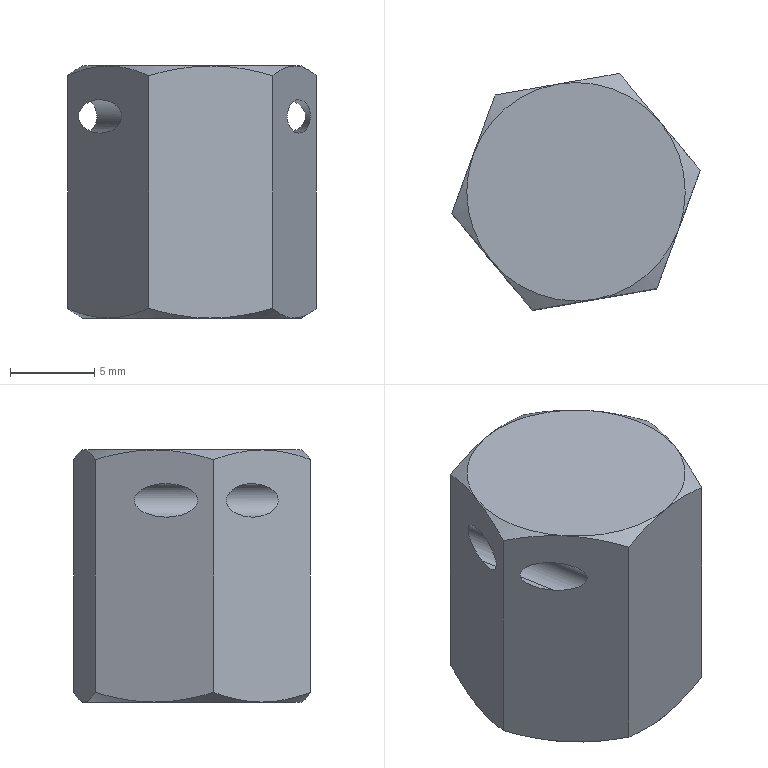Part | SolidWorks | features BaseBody 1 | 1 solid | 24 faces | box 14.79 x 14.092 x 15 mm | volume 2158 mm3 | cone 12 | plane 8 | cylinder 4 | commonest cylinder face diameters 2 x4
STEP:
#1=CARTESIAN_POINT('',(-50.82,56.44,-257.05));
#2=VERTEX_POINT('',#1);
#3=CARTESIAN_POINT('',(-50.82,56.44,-255.05));
#4=VERTEX_POINT('',#3);
#5=CARTESIAN_POINT('',(-50.82,56.44,-257.05));
#6=CARTESIAN_POINT('',(-49.442,60.195,-257.05));
#7=CARTESIAN_POINT('',(-49.442,60.195,-255.05));
#8=CARTESIAN_POINT('',(-50.82,56.44,-255.05));
#9=(BOUNDED_CURVE()B_SPLINE_CURVE(3,(#5,#6,#7,#8),.UNSPECIFIED.,.F.,.F.)B_SPLINE_CURVE_WITH_KNOTS((4,4),(1.571,4.712),.UNSPECIFIED.)CURVE()GEOMETRIC_REPRESENTATION_ITEM()RATIONAL_B_SPLINE_CURVE((1.,0.3333,0.3333,1.))REPRESENTATION_ITEM(''));
#10=EDGE_CURVE('',#2,#4,#9,.T.);
#11=ORIENTED_EDGE('',*,*,#10,.F.);
#12=CARTESIAN_POINT('',(-49.929,51.301,-257.05));
#13=VERTEX_POINT('',#12);
#14=CARTESIAN_POINT('',(-51.657,61.26,-257.05));
#15=DIRECTION('',(0.171,-0.9853,0.));
#16=VECTOR('',#15,1000.);
#17=LINE('',#14,#16);
#18=EDGE_CURVE('',#2,#13,#17,.T.);
#19=ORIENTED_EDGE('',*,*,#18,.T.);
#20=CARTESIAN_POINT('',(-49.929,51.301,-255.05));
#21=VERTEX_POINT('',#20);
#22=CARTESIAN_POINT('',(-49.929,51.301,-255.05));
#23=CARTESIAN_POINT('',(-47.366,48.23,-255.05));
#24=CARTESIAN_POINT('',(-47.366,48.23,-257.05));
#25=CARTESIAN_POINT('',(-49.929,51.301,-257.05));
#26=(BOUNDED_CURVE()B_SPLINE_CURVE(3,(#22,#23,#24,#25),.UNSPECIFIED.,.F.,.F.)B_SPLINE_CURVE_WITH_KNOTS((4,4),(4.712,7.854),.UNSPECIFIED.)CURVE()GEOMETRIC_REPRESENTATION_ITEM()RATIONAL_B_SPLINE_CURVE((1.,0.3333,0.3333,1.))REPRESENTATION_ITEM(''));
#27=EDGE_CURVE('',#21,#13,#26,.T.);
#28=ORIENTED_EDGE('',*,*,#27,.F.);
#29=CARTESIAN_POINT('',(-51.657,61.26,-255.05));
#30=DIRECTION('',(0.171,-0.9853,0.));
#31=VECTOR('',#30,1000.);
#32=LINE('',#29,#31);
#33=EDGE_CURVE('',#4,#21,#32,.T.);
#34=ORIENTED_EDGE('',*,*,#33,.F.);
#35=EDGE_LOOP('',(#11,#19,#28,#34));
#36=FACE_OUTER_BOUND('',#35,.T.);
#37=CARTESIAN_POINT('',(-51.657,61.26,-256.05));
#38=DIRECTION('',(0.171,-0.9853,0.));
#39=DIRECTION('',(0.,0.,1.));
#40=AXIS2_PLACEMENT_3D('',#37,#38,#39);
#41=CYLINDRICAL_SURFACE('',#40,1.);
#42=ADVANCED_FACE('',(#36),#41,.F.);
#43=CARTESIAN_POINT('',(-38.997,58.491,-257.05));
#44=VERTEX_POINT('',#43);
#45=CARTESIAN_POINT('',(-38.997,58.491,-255.05));
#46=VERTEX_POINT('',#45);
#47=CARTESIAN_POINT('',(-38.997,58.491,-257.05));
#48=CARTESIAN_POINT('',(-36.434,55.42,-257.05));
#49=CARTESIAN_POINT('',(-36.434,55.42,-255.05));
#50=CARTESIAN_POINT('',(-38.997,58.491,-255.05));
#51=(BOUNDED_CURVE()B_SPLINE_CURVE(3,(#47,#48,#49,#50),.UNSPECIFIED.,.F.,.F.)B_SPLINE_CURVE_WITH_KNOTS((4,4),(4.712,7.854),.UNSPECIFIED.)CURVE()GEOMETRIC_REPRESENTATION_ITEM()RATIONAL_B_SPLINE_CURVE((1.,0.3333,0.3333,1.))REPRESENTATION_ITEM(''));
#52=EDGE_CURVE('',#44,#46,#51,.T.);
#53=ORIENTED_EDGE('',*,*,#52,.F.);
#54=CARTESIAN_POINT('',(-38.105,53.353,-257.05));
#55=VERTEX_POINT('',#54);
#56=CARTESIAN_POINT('',(-39.833,63.312,-257.05));
#57=DIRECTION('',(0.171,-0.9853,0.));
#58=VECTOR('',#57,1000.);
#59=LINE('',#56,#58);
#60=EDGE_CURVE('',#44,#55,#59,.T.);
#61=ORIENTED_EDGE('',*,*,#60,.T.);
#62=CARTESIAN_POINT('',(-38.105,53.353,-255.05));
#63=VERTEX_POINT('',#62);
#64=CARTESIAN_POINT('',(-38.105,53.353,-255.05));
#65=CARTESIAN_POINT('',(-36.727,57.108,-255.05));
#66=CARTESIAN_POINT('',(-36.727,57.108,-257.05));
#67=CARTESIAN_POINT('',(-38.105,53.353,-257.05));
#68=(BOUNDED_CURVE()B_SPLINE_CURVE(3,(#64,#65,#66,#67),.UNSPECIFIED.,.F.,.F.)B_SPLINE_CURVE_WITH_KNOTS((4,4),(1.571,4.712),.UNSPECIFIED.)CURVE()GEOMETRIC_REPRESENTATION_ITEM()RATIONAL_B_SPLINE_CURVE((1.,0.3333,0.3333,1.))REPRESENTATION_ITEM(''));
#69=EDGE_CURVE('',#63,#55,#68,.T.);
#70=ORIENTED_EDGE('',*,*,#69,.F.);
#71=CARTESIAN_POINT('',(-39.833,63.312,-255.05));
#72=DIRECTION('',(0.171,-0.9853,0.));
#73=VECTOR('',#72,1000.);
#74=LINE('',#71,#73);
#75=EDGE_CURVE('',#46,#63,#74,.T.);
#76=ORIENTED_EDGE('',*,*,#75,.F.);
#77=EDGE_LOOP('',(#53,#61,#70,#76));
#78=FACE_OUTER_BOUND('',#77,.T.);
#79=CARTESIAN_POINT('',(-39.833,63.312,-256.05));
#80=DIRECTION('',(0.171,-0.9853,0.));
#81=DIRECTION('',(0.,0.,1.));
#82=AXIS2_PLACEMENT_3D('',#79,#80,#81);
#83=CYLINDRICAL_SURFACE('',#82,1.);
#84=ADVANCED_FACE('',(#78),#83,.F.);
#85=ORIENTED_EDGE('',*,*,#60,.F.);
#86=CARTESIAN_POINT('',(-38.997,58.491,-255.05));
#87=CARTESIAN_POINT('',(-41.56,61.562,-255.05));
#88=CARTESIAN_POINT('',(-41.56,61.562,-257.05));
#89=CARTESIAN_POINT('',(-38.997,58.491,-257.05));
#90=(BOUNDED_CURVE()B_SPLINE_CURVE(3,(#86,#87,#88,#89),.UNSPECIFIED.,.F.,.F.)B_SPLINE_CURVE_WITH_KNOTS((4,4),(1.571,4.712),.UNSPECIFIED.)CURVE()GEOMETRIC_REPRESENTATION_ITEM()RATIONAL_B_SPLINE_CURVE((1.,0.3333,0.3333,1.))REPRESENTATION_ITEM(''));
#91=EDGE_CURVE('',#46,#44,#90,.T.);
#92=ORIENTED_EDGE('',*,*,#91,.F.);
#93=ORIENTED_EDGE('',*,*,#75,.T.);
#94=CARTESIAN_POINT('',(-38.105,53.353,-257.05));
#95=CARTESIAN_POINT('',(-39.484,49.598,-257.05));
#96=CARTESIAN_POINT('',(-39.484,49.598,-255.05));
#97=CARTESIAN_POINT('',(-38.105,53.353,-255.05));
#98=(BOUNDED_CURVE()B_SPLINE_CURVE(3,(#94,#95,#96,#97),.UNSPECIFIED.,.F.,.F.)B_SPLINE_CURVE_WITH_KNOTS((4,4),(4.712,7.854),.UNSPECIFIED.)CURVE()GEOMETRIC_REPRESENTATION_ITEM()RATIONAL_B_SPLINE_CURVE((1.,0.3333,0.3333,1.))REPRESENTATION_ITEM(''));
#99=EDGE_CURVE('',#55,#63,#98,.T.);
#100=ORIENTED_EDGE('',*,*,#99,.F.);
#101=EDGE_LOOP('',(#85,#92,#93,#100));
#102=FACE_OUTER_BOUND('',#101,.T.);
#103=CARTESIAN_POINT('',(-39.833,63.312,-256.05));
#104=DIRECTION('',(0.171,-0.9853,0.));
#105=DIRECTION('',(0.,0.,1.));
#106=AXIS2_PLACEMENT_3D('',#103,#104,#105);
#107=CYLINDRICAL_SURFACE('',#106,1.);
#108=ADVANCED_FACE('',(#102),#107,.F.);
#109=ORIENTED_EDGE('',*,*,#18,.F.);
#110=CARTESIAN_POINT('',(-50.82,56.44,-255.05));
#111=CARTESIAN_POINT('',(-52.199,52.685,-255.05));
#112=CARTESIAN_POINT('',(-52.199,52.685,-257.05));
#113=CARTESIAN_POINT('',(-50.82,56.44,-257.05));
#114=(BOUNDED_CURVE()B_SPLINE_CURVE(3,(#110,#111,#112,#113),.UNSPECIFIED.,.F.,.F.)B_SPLINE_CURVE_WITH_KNOTS((4,4),(4.712,7.854),.UNSPECIFIED.)CURVE()GEOMETRIC_REPRESENTATION_ITEM()RATIONAL_B_SPLINE_CURVE((1.,0.3333,0.3333,1.))REPRESENTATION_ITEM(''));
#115=EDGE_CURVE('',#4,#2,#114,.T.);
#116=ORIENTED_EDGE('',*,*,#115,.F.);
#117=ORIENTED_EDGE('',*,*,#33,.T.);
#118=CARTESIAN_POINT('',(-49.929,51.301,-257.05));
#119=CARTESIAN_POINT('',(-52.492,54.372,-257.05));
#120=CARTESIAN_POINT('',(-52.492,54.372,-255.05));
#121=CARTESIAN_POINT('',(-49.929,51.301,-255.05));
#122=(BOUNDED_CURVE()B_SPLINE_CURVE(3,(#118,#119,#120,#121),.UNSPECIFIED.,.F.,.F.)B_SPLINE_CURVE_WITH_KNOTS((4,4),(1.571,4.712),.UNSPECIFIED.)CURVE()GEOMETRIC_REPRESENTATION_ITEM()RATIONAL_B_SPLINE_CURVE((1.,0.3333,0.3333,1.))REPRESENTATION_ITEM(''));
#123=EDGE_CURVE('',#13,#21,#122,.T.);
#124=ORIENTED_EDGE('',*,*,#123,.F.);
#125=EDGE_LOOP('',(#109,#116,#117,#124));
#126=FACE_OUTER_BOUND('',#125,.T.);
#127=CARTESIAN_POINT('',(-51.657,61.26,-256.05));
#128=DIRECTION('',(0.171,-0.9853,0.));
#129=DIRECTION('',(0.,0.,1.));
#130=AXIS2_PLACEMENT_3D('',#127,#128,#129);
#131=CYLINDRICAL_SURFACE('',#130,1.);
#132=ADVANCED_FACE('',(#126),#131,.F.);
#133=CARTESIAN_POINT('',(-45.574,61.301,-268.05));
#134=VERTEX_POINT('',#133);
#135=CARTESIAN_POINT('',(-50.565,57.136,-268.05));
#136=VERTEX_POINT('',#135);
#137=CARTESIAN_POINT('',(-44.463,54.896,-268.05));
#138=DIRECTION('',(0.,0.,1.));
#139=DIRECTION('',(-0.171,0.9853,0.));
#140=AXIS2_PLACEMENT_3D('',#137,#138,#139);
#141=CIRCLE('',#140,6.5);
#142=EDGE_CURVE('',#134,#136,#141,.T.);
#143=ORIENTED_EDGE('',*,*,#142,.F.);
#144=CARTESIAN_POINT('',(-39.472,59.061,-268.05));
#145=VERTEX_POINT('',#144);
#146=CARTESIAN_POINT('',(-44.463,54.896,-268.05));
#147=DIRECTION('',(0.,0.,1.));
#148=DIRECTION('',(-0.171,0.9853,0.));
#149=AXIS2_PLACEMENT_3D('',#146,#147,#148);
#150=CIRCLE('',#149,6.5);
#151=EDGE_CURVE('',#145,#134,#150,.T.);
#152=ORIENTED_EDGE('',*,*,#151,.F.);
#153=CARTESIAN_POINT('',(-38.361,52.656,-268.05));
#154=VERTEX_POINT('',#153);
#155=CARTESIAN_POINT('',(-44.463,54.896,-268.05));
#156=DIRECTION('',(0.,0.,1.));
#157=DIRECTION('',(-0.171,0.9853,0.));
#158=AXIS2_PLACEMENT_3D('',#155,#156,#157);
#159=CIRCLE('',#158,6.5);
#160=EDGE_CURVE('',#154,#145,#159,.T.);
#161=ORIENTED_EDGE('',*,*,#160,.F.);
#162=CARTESIAN_POINT('',(-43.352,48.492,-268.05));
#163=VERTEX_POINT('',#162);
#164=CARTESIAN_POINT('',(-44.463,54.896,-268.05));
#165=DIRECTION('',(0.,0.,1.));
#166=DIRECTION('',(-0.171,0.9853,0.));
#167=AXIS2_PLACEMENT_3D('',#164,#165,#166);
#168=CIRCLE('',#167,6.5);
#169=EDGE_CURVE('',#163,#154,#168,.T.);
#170=ORIENTED_EDGE('',*,*,#169,.F.);
#171=CARTESIAN_POINT('',(-49.454,50.732,-268.05));
#172=VERTEX_POINT('',#171);
#173=CARTESIAN_POINT('',(-44.463,54.896,-268.05));
#174=DIRECTION('',(0.,0.,1.));
#175=DIRECTION('',(-0.171,0.9853,0.));
#176=AXIS2_PLACEMENT_3D('',#173,#174,#175);
#177=CIRCLE('',#176,6.5);
#178=EDGE_CURVE('',#172,#163,#177,.T.);
#179=ORIENTED_EDGE('',*,*,#178,.F.);
#180=CARTESIAN_POINT('',(-44.463,54.896,-268.05));
#181=DIRECTION('',(0.,0.,1.));
#182=DIRECTION('',(-0.171,0.9853,0.));
#183=AXIS2_PLACEMENT_3D('',#180,#181,#182);
#184=CIRCLE('',#183,6.5);
#185=EDGE_CURVE('',#136,#172,#184,.T.);
#186=ORIENTED_EDGE('',*,*,#185,.F.);
#187=EDGE_LOOP('',(#143,#152,#161,#170,#179,#186));
#188=FACE_OUTER_BOUND('',#187,.T.);
#189=CARTESIAN_POINT('',(-42.24,42.088,-268.05));
#190=DIRECTION('',(0.,0.,1.));
#191=DIRECTION('',(0.,-1.,0.));
#192=AXIS2_PLACEMENT_3D('',#189,#190,#191);
#193=PLANE('',#192);
#194=ADVANCED_FACE('',(#188),#193,.F.);
#195=CARTESIAN_POINT('',(-49.272,60.659,-267.469));
#196=VERTEX_POINT('',#195);
#197=CARTESIAN_POINT('',(-50.565,57.136,-268.05));
#198=CARTESIAN_POINT('',(-50.123,58.338,-268.05));
#199=CARTESIAN_POINT('',(-49.694,59.508,-267.823));
#200=CARTESIAN_POINT('',(-49.272,60.659,-267.469));
#201=B_SPLINE_CURVE_WITH_KNOTS('',3,(#197,#198,#199,#200),.UNSPECIFIED.,.F.,.F.,(4,4),(0.,0.003797),.UNSPECIFIED.);
#202=EDGE_CURVE('',#136,#196,#201,.T.);
#203=ORIENTED_EDGE('',*,*,#202,.T.);
#204=CARTESIAN_POINT('',(-49.272,60.659,-267.469));
#205=CARTESIAN_POINT('',(-48.064,60.869,-267.823));
#206=CARTESIAN_POINT('',(-46.836,61.082,-268.05));
#207=CARTESIAN_POINT('',(-45.574,61.301,-268.05));
#208=B_SPLINE_CURVE_WITH_KNOTS('',3,(#204,#205,#206,#207),.UNSPECIFIED.,.F.,.F.,(4,4),(0.,0.003797),.UNSPECIFIED.);
#209=EDGE_CURVE('',#196,#134,#208,.T.);
#210=ORIENTED_EDGE('',*,*,#209,.T.);
#211=ORIENTED_EDGE('',*,*,#142,.T.);
#212=EDGE_LOOP('',(#203,#210,#211));
#213=FACE_OUTER_BOUND('',#212,.T.);
#214=CARTESIAN_POINT('',(-44.463,54.896,-265.401));
#215=DIRECTION('',(0.,0.,1.));
#216=DIRECTION('',(-0.171,0.9853,0.));
#217=AXIS2_PLACEMENT_3D('',#214,#215,#216);
#218=CONICAL_SURFACE('',#217,11.087,1.047);
#219=ADVANCED_FACE('',(#213),#218,.T.);
#220=CARTESIAN_POINT('',(-51.858,53.613,-267.469));
#221=VERTEX_POINT('',#220);
#222=CARTESIAN_POINT('',(-49.454,50.732,-268.05));
#223=CARTESIAN_POINT('',(-50.274,51.715,-268.05));
#224=CARTESIAN_POINT('',(-51.072,52.672,-267.823));
#225=CARTESIAN_POINT('',(-51.858,53.613,-267.469));
#226=B_SPLINE_CURVE_WITH_KNOTS('',3,(#222,#223,#224,#225),.UNSPECIFIED.,.F.,.F.,(4,4),(0.,0.003797),.UNSPECIFIED.);
#227=EDGE_CURVE('',#172,#221,#226,.T.);
#228=ORIENTED_EDGE('',*,*,#227,.T.);
#229=CARTESIAN_POINT('',(-51.858,53.613,-267.469));
#230=CARTESIAN_POINT('',(-51.435,54.764,-267.823));
#231=CARTESIAN_POINT('',(-51.006,55.934,-268.05));
#232=CARTESIAN_POINT('',(-50.565,57.136,-268.05));
#233=B_SPLINE_CURVE_WITH_KNOTS('',3,(#229,#230,#231,#232),.UNSPECIFIED.,.F.,.F.,(4,4),(0.,0.003797),.UNSPECIFIED.);
#234=EDGE_CURVE('',#221,#136,#233,.T.);
#235=ORIENTED_EDGE('',*,*,#234,.T.);
#236=ORIENTED_EDGE('',*,*,#185,.T.);
#237=EDGE_LOOP('',(#228,#235,#236));
#238=FACE_OUTER_BOUND('',#237,.T.);
#239=CARTESIAN_POINT('',(-44.463,54.896,-265.401));
#240=DIRECTION('',(0.,0.,1.));
#241=DIRECTION('',(-0.171,0.9853,0.));
#242=AXIS2_PLACEMENT_3D('',#239,#240,#241);
#243=CONICAL_SURFACE('',#242,11.087,1.047);
#244=ADVANCED_FACE('',(#238),#243,.T.);
#245=CARTESIAN_POINT('',(-47.049,47.85,-267.469));
#246=VERTEX_POINT('',#245);
#247=CARTESIAN_POINT('',(-47.049,47.85,-267.469));
#248=CARTESIAN_POINT('',(-47.835,48.792,-267.823));
#249=CARTESIAN_POINT('',(-48.633,49.748,-268.05));
#250=CARTESIAN_POINT('',(-49.454,50.732,-268.05));
#251=B_SPLINE_CURVE_WITH_KNOTS('',3,(#247,#248,#249,#250),.UNSPECIFIED.,.F.,.F.,(4,4),(0.,0.003797),.UNSPECIFIED.);
#252=EDGE_CURVE('',#246,#172,#251,.T.);
#253=ORIENTED_EDGE('',*,*,#252,.T.);
#254=ORIENTED_EDGE('',*,*,#178,.T.);
#255=CARTESIAN_POINT('',(-43.352,48.492,-268.05));
#256=CARTESIAN_POINT('',(-44.614,48.273,-268.05));
#257=CARTESIAN_POINT('',(-45.841,48.06,-267.823));
#258=CARTESIAN_POINT('',(-47.049,47.85,-267.469));
#259=B_SPLINE_CURVE_WITH_KNOTS('',3,(#255,#256,#257,#258),.UNSPECIFIED.,.F.,.F.,(4,4),(0.,0.003797),.UNSPECIFIED.);
#260=EDGE_CURVE('',#163,#246,#259,.T.);
#261=ORIENTED_EDGE('',*,*,#260,.T.);
#262=EDGE_LOOP('',(#253,#254,#261));
#263=FACE_OUTER_BOUND('',#262,.T.);
#264=CARTESIAN_POINT('',(-44.463,54.896,-265.401));
#265=DIRECTION('',(0.,0.,1.));
#266=DIRECTION('',(-0.171,0.9853,0.));
#267=AXIS2_PLACEMENT_3D('',#264,#265,#266);
#268=CONICAL_SURFACE('',#267,11.087,1.047);
#269=ADVANCED_FACE('',(#263),#268,.T.);
#270=CARTESIAN_POINT('',(-39.654,49.134,-267.469));
#271=VERTEX_POINT('',#270);
#272=CARTESIAN_POINT('',(-38.361,52.656,-268.05));
#273=CARTESIAN_POINT('',(-38.802,51.454,-268.05));
#274=CARTESIAN_POINT('',(-39.232,50.285,-267.823));
#275=CARTESIAN_POINT('',(-39.654,49.134,-267.469));
#276=B_SPLINE_CURVE_WITH_KNOTS('',3,(#272,#273,#274,#275),.UNSPECIFIED.,.F.,.F.,(4,4),(0.,0.003797),.UNSPECIFIED.);
#277=EDGE_CURVE('',#154,#271,#276,.T.);
#278=ORIENTED_EDGE('',*,*,#277,.T.);
#279=CARTESIAN_POINT('',(-39.654,49.134,-267.469));
#280=CARTESIAN_POINT('',(-40.862,48.924,-267.823));
#281=CARTESIAN_POINT('',(-42.09,48.711,-268.05));
#282=CARTESIAN_POINT('',(-43.352,48.492,-268.05));
#283=B_SPLINE_CURVE_WITH_KNOTS('',3,(#279,#280,#281,#282),.UNSPECIFIED.,.F.,.F.,(4,4),(0.,0.003797),.UNSPECIFIED.);
#284=EDGE_CURVE('',#271,#163,#283,.T.);
#285=ORIENTED_EDGE('',*,*,#284,.T.);
#286=ORIENTED_EDGE('',*,*,#169,.T.);
#287=EDGE_LOOP('',(#278,#285,#286));
#288=FACE_OUTER_BOUND('',#287,.T.);
#289=CARTESIAN_POINT('',(-44.463,54.896,-265.401));
#290=DIRECTION('',(0.,0.,1.));
#291=DIRECTION('',(-0.171,0.9853,0.));
#292=AXIS2_PLACEMENT_3D('',#289,#290,#291);
#293=CONICAL_SURFACE('',#292,11.087,1.047);
#294=ADVANCED_FACE('',(#288),#293,.T.);
#295=CARTESIAN_POINT('',(-37.068,56.179,-267.469));
#296=VERTEX_POINT('',#295);
#297=CARTESIAN_POINT('',(-39.472,59.061,-268.05));
#298=CARTESIAN_POINT('',(-38.652,58.077,-268.05));
#299=CARTESIAN_POINT('',(-37.853,57.121,-267.823));
#300=CARTESIAN_POINT('',(-37.068,56.179,-267.469));
#301=B_SPLINE_CURVE_WITH_KNOTS('',3,(#297,#298,#299,#300),.UNSPECIFIED.,.F.,.F.,(4,4),(0.,0.003797),.UNSPECIFIED.);
#302=EDGE_CURVE('',#145,#296,#301,.T.);
#303=ORIENTED_EDGE('',*,*,#302,.T.);
#304=CARTESIAN_POINT('',(-37.068,56.179,-267.469));
#305=CARTESIAN_POINT('',(-37.49,55.028,-267.823));
#306=CARTESIAN_POINT('',(-37.92,53.859,-268.05));
#307=CARTESIAN_POINT('',(-38.361,52.656,-268.05));
#308=B_SPLINE_CURVE_WITH_KNOTS('',3,(#304,#305,#306,#307),.UNSPECIFIED.,.F.,.F.,(4,4),(0.,0.003797),.UNSPECIFIED.);
#309=EDGE_CURVE('',#296,#154,#308,.T.);
#310=ORIENTED_EDGE('',*,*,#309,.T.);
#311=ORIENTED_EDGE('',*,*,#160,.T.);
#312=EDGE_LOOP('',(#303,#310,#311));
#313=FACE_OUTER_BOUND('',#312,.T.);
#314=CARTESIAN_POINT('',(-44.463,54.896,-265.401));
#315=DIRECTION('',(0.,0.,1.));
#316=DIRECTION('',(-0.171,0.9853,0.));
#317=AXIS2_PLACEMENT_3D('',#314,#315,#316);
#318=CONICAL_SURFACE('',#317,11.087,1.047);
#319=ADVANCED_FACE('',(#313),#318,.T.);
#320=CARTESIAN_POINT('',(-41.877,61.942,-267.469));
#321=VERTEX_POINT('',#320);
#322=CARTESIAN_POINT('',(-45.574,61.301,-268.05));
#323=CARTESIAN_POINT('',(-44.312,61.52,-268.05));
#324=CARTESIAN_POINT('',(-43.085,61.732,-267.823));
#325=CARTESIAN_POINT('',(-41.877,61.942,-267.469));
#326=B_SPLINE_CURVE_WITH_KNOTS('',3,(#322,#323,#324,#325),.UNSPECIFIED.,.F.,.F.,(4,4),(0.,0.003797),.UNSPECIFIED.);
#327=EDGE_CURVE('',#134,#321,#326,.T.);
#328=ORIENTED_EDGE('',*,*,#327,.T.);
#329=CARTESIAN_POINT('',(-41.877,61.942,-267.469));
#330=CARTESIAN_POINT('',(-41.091,61.001,-267.823));
#331=CARTESIAN_POINT('',(-40.293,60.044,-268.05));
#332=CARTESIAN_POINT('',(-39.472,59.061,-268.05));
#333=B_SPLINE_CURVE_WITH_KNOTS('',3,(#329,#330,#331,#332),.UNSPECIFIED.,.F.,.F.,(4,4),(0.,0.003797),.UNSPECIFIED.);
#334=EDGE_CURVE('',#321,#145,#333,.T.);
#335=ORIENTED_EDGE('',*,*,#334,.T.);
#336=ORIENTED_EDGE('',*,*,#151,.T.);
#337=EDGE_LOOP('',(#328,#335,#336));
#338=FACE_OUTER_BOUND('',#337,.T.);
#339=CARTESIAN_POINT('',(-44.463,54.896,-265.401));
#340=DIRECTION('',(0.,0.,1.));
#341=DIRECTION('',(-0.171,0.9853,0.));
#342=AXIS2_PLACEMENT_3D('',#339,#340,#341);
#343=CONICAL_SURFACE('',#342,11.087,1.047);
#344=ADVANCED_FACE('',(#338),#343,.T.);
#345=CARTESIAN_POINT('',(-39.472,59.061,-253.05));
#346=VERTEX_POINT('',#345);
#347=CARTESIAN_POINT('',(-45.574,61.301,-253.05));
#348=VERTEX_POINT('',#347);
#349=CARTESIAN_POINT('',(-44.463,54.896,-253.05));
#350=DIRECTION('',(0.,0.,1.));
#351=DIRECTION('',(-0.171,0.9853,0.));
#352=AXIS2_PLACEMENT_3D('',#349,#350,#351);
#353=CIRCLE('',#352,6.5);
#354=EDGE_CURVE('',#346,#348,#353,.T.);
#355=ORIENTED_EDGE('',*,*,#354,.T.);
#356=CARTESIAN_POINT('',(-50.565,57.136,-253.05));
#357=VERTEX_POINT('',#356);
#358=CARTESIAN_POINT('',(-44.463,54.896,-253.05));
#359=DIRECTION('',(0.,0.,1.));
#360=DIRECTION('',(-0.171,0.9853,0.));
#361=AXIS2_PLACEMENT_3D('',#358,#359,#360);
#362=CIRCLE('',#361,6.5);
#363=EDGE_CURVE('',#348,#357,#362,.T.);
#364=ORIENTED_EDGE('',*,*,#363,.T.);
#365=CARTESIAN_POINT('',(-49.454,50.732,-253.05));
#366=VERTEX_POINT('',#365);
#367=CARTESIAN_POINT('',(-44.463,54.896,-253.05));
#368=DIRECTION('',(0.,0.,1.));
#369=DIRECTION('',(-0.171,0.9853,0.));
#370=AXIS2_PLACEMENT_3D('',#367,#368,#369);
#371=CIRCLE('',#370,6.5);
#372=EDGE_CURVE('',#357,#366,#371,.T.);
#373=ORIENTED_EDGE('',*,*,#372,.T.);
#374=CARTESIAN_POINT('',(-43.352,48.492,-253.05));
#375=VERTEX_POINT('',#374);
#376=CARTESIAN_POINT('',(-44.463,54.896,-253.05));
#377=DIRECTION('',(0.,0.,1.));
#378=DIRECTION('',(-0.171,0.9853,0.));
#379=AXIS2_PLACEMENT_3D('',#376,#377,#378);
#380=CIRCLE('',#379,6.5);
#381=EDGE_CURVE('',#366,#375,#380,.T.);
#382=ORIENTED_EDGE('',*,*,#381,.T.);
#383=CARTESIAN_POINT('',(-38.361,52.656,-253.05));
#384=VERTEX_POINT('',#383);
#385=CARTESIAN_POINT('',(-44.463,54.896,-253.05));
#386=DIRECTION('',(0.,0.,1.));
#387=DIRECTION('',(-0.171,0.9853,0.));
#388=AXIS2_PLACEMENT_3D('',#385,#386,#387);
#389=CIRCLE('',#388,6.5);
#390=EDGE_CURVE('',#375,#384,#389,.T.);
#391=ORIENTED_EDGE('',*,*,#390,.T.);
#392=CARTESIAN_POINT('',(-44.463,54.896,-253.05));
#393=DIRECTION('',(0.,0.,1.));
#394=DIRECTION('',(-0.171,0.9853,0.));
#395=AXIS2_PLACEMENT_3D('',#392,#393,#394);
#396=CIRCLE('',#395,6.5);
#397=EDGE_CURVE('',#384,#346,#396,.T.);
#398=ORIENTED_EDGE('',*,*,#397,.T.);
#399=EDGE_LOOP('',(#355,#364,#373,#382,#391,#398));
#400=FACE_OUTER_BOUND('',#399,.T.);
#401=CARTESIAN_POINT('',(-42.24,42.088,-253.05));
#402=DIRECTION('',(0.,0.,1.));
#403=DIRECTION('',(0.,-1.,0.));
#404=AXIS2_PLACEMENT_3D('',#401,#402,#403);
#405=PLANE('',#404);
#406=ADVANCED_FACE('',(#400),#405,.T.);
#407=CARTESIAN_POINT('',(-49.272,60.659,-253.631));
#408=VERTEX_POINT('',#407);
#409=CARTESIAN_POINT('',(-45.574,61.301,-253.05));
#410=CARTESIAN_POINT('',(-46.836,61.082,-253.05));
#411=CARTESIAN_POINT('',(-48.064,60.869,-253.277));
#412=CARTESIAN_POINT('',(-49.272,60.659,-253.631));
#413=B_SPLINE_CURVE_WITH_KNOTS('',3,(#409,#410,#411,#412),.UNSPECIFIED.,.F.,.F.,(4,4),(0.,0.003797),.UNSPECIFIED.);
#414=EDGE_CURVE('',#348,#408,#413,.T.);
#415=ORIENTED_EDGE('',*,*,#414,.T.);
#416=CARTESIAN_POINT('',(-49.272,60.659,-253.631));
#417=CARTESIAN_POINT('',(-49.694,59.508,-253.277));
#418=CARTESIAN_POINT('',(-50.123,58.338,-253.05));
#419=CARTESIAN_POINT('',(-50.565,57.136,-253.05));
#420=B_SPLINE_CURVE_WITH_KNOTS('',3,(#416,#417,#418,#419),.UNSPECIFIED.,.F.,.F.,(4,4),(0.,0.003797),.UNSPECIFIED.);
#421=EDGE_CURVE('',#408,#357,#420,.T.);
#422=ORIENTED_EDGE('',*,*,#421,.T.);
#423=ORIENTED_EDGE('',*,*,#363,.F.);
#424=EDGE_LOOP('',(#415,#422,#423));
#425=FACE_OUTER_BOUND('',#424,.T.);
#426=CARTESIAN_POINT('',(-44.463,54.896,-253.05));
#427=DIRECTION('',(0.,0.,-1.));
#428=DIRECTION('',(0.171,-0.9853,0.));
#429=AXIS2_PLACEMENT_3D('',#426,#427,#428);
#430=CONICAL_SURFACE('',#429,6.5,1.047);
#431=ADVANCED_FACE('',(#425),#430,.T.);
#432=CARTESIAN_POINT('',(-51.858,53.613,-253.631));
#433=VERTEX_POINT('',#432);
#434=CARTESIAN_POINT('',(-50.565,57.136,-253.05));
#435=CARTESIAN_POINT('',(-51.006,55.934,-253.05));
#436=CARTESIAN_POINT('',(-51.435,54.764,-253.277));
#437=CARTESIAN_POINT('',(-51.858,53.613,-253.631));
#438=B_SPLINE_CURVE_WITH_KNOTS('',3,(#434,#435,#436,#437),.UNSPECIFIED.,.F.,.F.,(4,4),(0.,0.003797),.UNSPECIFIED.);
#439=EDGE_CURVE('',#357,#433,#438,.T.);
#440=ORIENTED_EDGE('',*,*,#439,.T.);
#441=CARTESIAN_POINT('',(-51.858,53.613,-253.631));
#442=CARTESIAN_POINT('',(-51.072,52.672,-253.277));
#443=CARTESIAN_POINT('',(-50.274,51.715,-253.05));
#444=CARTESIAN_POINT('',(-49.454,50.732,-253.05));
#445=B_SPLINE_CURVE_WITH_KNOTS('',3,(#441,#442,#443,#444),.UNSPECIFIED.,.F.,.F.,(4,4),(0.,0.003797),.UNSPECIFIED.);
#446=EDGE_CURVE('',#433,#366,#445,.T.);
#447=ORIENTED_EDGE('',*,*,#446,.T.);
#448=ORIENTED_EDGE('',*,*,#372,.F.);
#449=EDGE_LOOP('',(#440,#447,#448));
#450=FACE_OUTER_BOUND('',#449,.T.);
#451=CARTESIAN_POINT('',(-44.463,54.896,-253.05));
#452=DIRECTION('',(0.,0.,-1.));
#453=DIRECTION('',(0.171,-0.9853,0.));
#454=AXIS2_PLACEMENT_3D('',#451,#452,#453);
#455=CONICAL_SURFACE('',#454,6.5,1.047);
#456=ADVANCED_FACE('',(#450),#455,.T.);
#457=CARTESIAN_POINT('',(-47.049,47.85,-253.631));
#458=VERTEX_POINT('',#457);
#459=CARTESIAN_POINT('',(-49.454,50.732,-253.05));
#460=CARTESIAN_POINT('',(-48.633,49.748,-253.05));
#461=CARTESIAN_POINT('',(-47.835,48.792,-253.277));
#462=CARTESIAN_POINT('',(-47.049,47.85,-253.631));
#463=B_SPLINE_CURVE_WITH_KNOTS('',3,(#459,#460,#461,#462),.UNSPECIFIED.,.F.,.F.,(4,4),(0.,0.003797),.UNSPECIFIED.);
#464=EDGE_CURVE('',#366,#458,#463,.T.);
#465=ORIENTED_EDGE('',*,*,#464,.T.);
#466=CARTESIAN_POINT('',(-47.049,47.85,-253.631));
#467=CARTESIAN_POINT('',(-45.841,48.06,-253.277));
#468=CARTESIAN_POINT('',(-44.614,48.273,-253.05));
#469=CARTESIAN_POINT('',(-43.352,48.492,-253.05));
#470=B_SPLINE_CURVE_WITH_KNOTS('',3,(#466,#467,#468,#469),.UNSPECIFIED.,.F.,.F.,(4,4),(0.,0.003797),.UNSPECIFIED.);
#471=EDGE_CURVE('',#458,#375,#470,.T.);
#472=ORIENTED_EDGE('',*,*,#471,.T.);
#473=ORIENTED_EDGE('',*,*,#381,.F.);
#474=EDGE_LOOP('',(#465,#472,#473));
#475=FACE_OUTER_BOUND('',#474,.T.);
#476=CARTESIAN_POINT('',(-44.463,54.896,-253.05));
#477=DIRECTION('',(0.,0.,-1.));
#478=DIRECTION('',(0.171,-0.9853,0.));
#479=AXIS2_PLACEMENT_3D('',#476,#477,#478);
#480=CONICAL_SURFACE('',#479,6.5,1.047);
#481=ADVANCED_FACE('',(#475),#480,.T.);
#482=CARTESIAN_POINT('',(-39.654,49.134,-253.631));
#483=VERTEX_POINT('',#482);
#484=CARTESIAN_POINT('',(-39.654,49.134,-253.631));
#485=CARTESIAN_POINT('',(-39.232,50.285,-253.277));
#486=CARTESIAN_POINT('',(-38.802,51.454,-253.05));
#487=CARTESIAN_POINT('',(-38.361,52.656,-253.05));
#488=B_SPLINE_CURVE_WITH_KNOTS('',3,(#484,#485,#486,#487),.UNSPECIFIED.,.F.,.F.,(4,4),(0.,0.003797),.UNSPECIFIED.);
#489=EDGE_CURVE('',#483,#384,#488,.T.);
#490=ORIENTED_EDGE('',*,*,#489,.T.);
#491=ORIENTED_EDGE('',*,*,#390,.F.);
#492=CARTESIAN_POINT('',(-43.352,48.492,-253.05));
#493=CARTESIAN_POINT('',(-42.09,48.711,-253.05));
#494=CARTESIAN_POINT('',(-40.862,48.924,-253.277));
#495=CARTESIAN_POINT('',(-39.654,49.134,-253.631));
#496=B_SPLINE_CURVE_WITH_KNOTS('',3,(#492,#493,#494,#495),.UNSPECIFIED.,.F.,.F.,(4,4),(0.,0.003797),.UNSPECIFIED.);
#497=EDGE_CURVE('',#375,#483,#496,.T.);
#498=ORIENTED_EDGE('',*,*,#497,.T.);
#499=EDGE_LOOP('',(#490,#491,#498));
#500=FACE_OUTER_BOUND('',#499,.T.);
#501=CARTESIAN_POINT('',(-44.463,54.896,-253.05));
#502=DIRECTION('',(0.,0.,-1.));
#503=DIRECTION('',(0.171,-0.9853,0.));
#504=AXIS2_PLACEMENT_3D('',#501,#502,#503);
#505=CONICAL_SURFACE('',#504,6.5,1.047);
#506=ADVANCED_FACE('',(#500),#505,.T.);
#507=CARTESIAN_POINT('',(-37.068,56.179,-253.631));
#508=VERTEX_POINT('',#507);
#509=CARTESIAN_POINT('',(-37.068,56.179,-253.631));
#510=CARTESIAN_POINT('',(-37.853,57.121,-253.277));
#511=CARTESIAN_POINT('',(-38.652,58.077,-253.05));
#512=CARTESIAN_POINT('',(-39.472,59.061,-253.05));
#513=B_SPLINE_CURVE_WITH_KNOTS('',3,(#509,#510,#511,#512),.UNSPECIFIED.,.F.,.F.,(4,4),(0.,0.003797),.UNSPECIFIED.);
#514=EDGE_CURVE('',#508,#346,#513,.T.);
#515=ORIENTED_EDGE('',*,*,#514,.T.);
#516=ORIENTED_EDGE('',*,*,#397,.F.);
#517=CARTESIAN_POINT('',(-38.361,52.656,-253.05));
#518=CARTESIAN_POINT('',(-37.92,53.859,-253.05));
#519=CARTESIAN_POINT('',(-37.49,55.028,-253.277));
#520=CARTESIAN_POINT('',(-37.068,56.179,-253.631));
#521=B_SPLINE_CURVE_WITH_KNOTS('',3,(#517,#518,#519,#520),.UNSPECIFIED.,.F.,.F.,(4,4),(0.,0.003797),.UNSPECIFIED.);
#522=EDGE_CURVE('',#384,#508,#521,.T.);
#523=ORIENTED_EDGE('',*,*,#522,.T.);
#524=EDGE_LOOP('',(#515,#516,#523));
#525=FACE_OUTER_BOUND('',#524,.T.);
#526=CARTESIAN_POINT('',(-44.463,54.896,-253.05));
#527=DIRECTION('',(0.,0.,-1.));
#528=DIRECTION('',(0.171,-0.9853,0.));
#529=AXIS2_PLACEMENT_3D('',#526,#527,#528);
#530=CONICAL_SURFACE('',#529,6.5,1.047);
#531=ADVANCED_FACE('',(#525),#530,.T.);
#532=CARTESIAN_POINT('',(-41.877,61.942,-253.631));
#533=VERTEX_POINT('',#532);
#534=CARTESIAN_POINT('',(-41.877,61.942,-253.631));
#535=CARTESIAN_POINT('',(-43.085,61.732,-253.277));
#536=CARTESIAN_POINT('',(-44.312,61.52,-253.05));
#537=CARTESIAN_POINT('',(-45.574,61.301,-253.05));
#538=B_SPLINE_CURVE_WITH_KNOTS('',3,(#534,#535,#536,#537),.UNSPECIFIED.,.F.,.F.,(4,4),(0.,0.003797),.UNSPECIFIED.);
#539=EDGE_CURVE('',#533,#348,#538,.T.);
#540=ORIENTED_EDGE('',*,*,#539,.T.);
#541=ORIENTED_EDGE('',*,*,#354,.F.);
#542=CARTESIAN_POINT('',(-39.472,59.061,-253.05));
#543=CARTESIAN_POINT('',(-40.293,60.044,-253.05));
#544=CARTESIAN_POINT('',(-41.091,61.001,-253.277));
#545=CARTESIAN_POINT('',(-41.877,61.942,-253.631));
#546=B_SPLINE_CURVE_WITH_KNOTS('',3,(#542,#543,#544,#545),.UNSPECIFIED.,.F.,.F.,(4,4),(0.,0.003797),.UNSPECIFIED.);
#547=EDGE_CURVE('',#346,#533,#546,.T.);
#548=ORIENTED_EDGE('',*,*,#547,.T.);
#549=EDGE_LOOP('',(#540,#541,#548));
#550=FACE_OUTER_BOUND('',#549,.T.);
#551=CARTESIAN_POINT('',(-44.463,54.896,-253.05));
#552=DIRECTION('',(0.,0.,-1.));
#553=DIRECTION('',(0.171,-0.9853,0.));
#554=AXIS2_PLACEMENT_3D('',#551,#552,#553);
#555=CONICAL_SURFACE('',#554,6.5,1.047);
#556=ADVANCED_FACE('',(#550),#555,.T.);
#557=ORIENTED_EDGE('',*,*,#284,.F.);
#558=CARTESIAN_POINT('',(-39.654,49.134,-268.05));
#559=DIRECTION('',(0.,0.,1.));
#560=VECTOR('',#559,1000.);
#561=LINE('',#558,#560);
#562=EDGE_CURVE('',#271,#483,#561,.T.);
#563=ORIENTED_EDGE('',*,*,#562,.T.);
#564=ORIENTED_EDGE('',*,*,#497,.F.);
#565=ORIENTED_EDGE('',*,*,#471,.F.);
#566=CARTESIAN_POINT('',(-47.049,47.85,-268.05));
#567=DIRECTION('',(0.,0.,1.));
#568=VECTOR('',#567,1000.);
#569=LINE('',#566,#568);
#570=EDGE_CURVE('',#246,#458,#569,.T.);
#571=ORIENTED_EDGE('',*,*,#570,.F.);
#572=ORIENTED_EDGE('',*,*,#260,.F.);
#573=EDGE_LOOP('',(#557,#563,#564,#565,#571,#572));
#574=FACE_OUTER_BOUND('',#573,.T.);
#575=CARTESIAN_POINT('',(-39.654,49.134,-268.05));
#576=DIRECTION('',(-0.171,0.9853,0.));
#577=DIRECTION('',(0.,0.,1.));
#578=AXIS2_PLACEMENT_3D('',#575,#576,#577);
#579=PLANE('',#578);
#580=ADVANCED_FACE('',(#574),#579,.F.);
#581=ORIENTED_EDGE('',*,*,#309,.F.);
#582=CARTESIAN_POINT('',(-37.068,56.179,-268.05));
#583=DIRECTION('',(0.,0.,1.));
#584=VECTOR('',#583,1000.);
#585=LINE('',#582,#584);
#586=EDGE_CURVE('',#296,#508,#585,.T.);
#587=ORIENTED_EDGE('',*,*,#586,.T.);
#588=ORIENTED_EDGE('',*,*,#522,.F.);
#589=ORIENTED_EDGE('',*,*,#489,.F.);
#590=ORIENTED_EDGE('',*,*,#562,.F.);
#591=ORIENTED_EDGE('',*,*,#277,.F.);
#592=EDGE_LOOP('',(#581,#587,#588,#589,#590,#591));
#593=FACE_OUTER_BOUND('',#592,.T.);
#594=ORIENTED_EDGE('',*,*,#69,.T.);
#595=ORIENTED_EDGE('',*,*,#99,.T.);
#596=EDGE_LOOP('',(#594,#595));
#597=FACE_BOUND('',#596,.T.);
#598=CARTESIAN_POINT('',(-37.068,56.179,-268.05));
#599=DIRECTION('',(-0.9388,0.3446,0.));
#600=DIRECTION('',(0.,0.,1.));
#601=AXIS2_PLACEMENT_3D('',#598,#599,#600);
#602=PLANE('',#601);
#603=ADVANCED_FACE('',(#593,#597),#602,.F.);
#604=ORIENTED_EDGE('',*,*,#334,.F.);
#605=CARTESIAN_POINT('',(-41.877,61.942,-268.05));
#606=DIRECTION('',(0.,0.,1.));
#607=VECTOR('',#606,1000.);
#608=LINE('',#605,#607);
#609=EDGE_CURVE('',#321,#533,#608,.T.);
#610=ORIENTED_EDGE('',*,*,#609,.T.);
#611=ORIENTED_EDGE('',*,*,#547,.F.);
#612=ORIENTED_EDGE('',*,*,#514,.F.);
#613=ORIENTED_EDGE('',*,*,#586,.F.);
#614=ORIENTED_EDGE('',*,*,#302,.F.);
#615=EDGE_LOOP('',(#604,#610,#611,#612,#613,#614));
#616=FACE_OUTER_BOUND('',#615,.T.);
#617=ORIENTED_EDGE('',*,*,#91,.T.);
#618=ORIENTED_EDGE('',*,*,#52,.T.);
#619=EDGE_LOOP('',(#617,#618));
#620=FACE_BOUND('',#619,.T.);
#621=CARTESIAN_POINT('',(-41.877,61.942,-268.05));
#622=DIRECTION('',(-0.7678,-0.6407,0.));
#623=DIRECTION('',(-0.6407,0.7678,0.));
#624=AXIS2_PLACEMENT_3D('',#621,#622,#623);
#625=PLANE('',#624);
#626=ADVANCED_FACE('',(#616,#620),#625,.F.);
#627=ORIENTED_EDGE('',*,*,#209,.F.);
#628=CARTESIAN_POINT('',(-49.272,60.659,-268.05));
#629=DIRECTION('',(0.,0.,1.));
#630=VECTOR('',#629,1000.);
#631=LINE('',#628,#630);
#632=EDGE_CURVE('',#196,#408,#631,.T.);
#633=ORIENTED_EDGE('',*,*,#632,.T.);
#634=ORIENTED_EDGE('',*,*,#414,.F.);
#635=ORIENTED_EDGE('',*,*,#539,.F.);
#636=ORIENTED_EDGE('',*,*,#609,.F.);
#637=ORIENTED_EDGE('',*,*,#327,.F.);
#638=EDGE_LOOP('',(#627,#633,#634,#635,#636,#637));
#639=FACE_OUTER_BOUND('',#638,.T.);
#640=CARTESIAN_POINT('',(-49.272,60.659,-268.05));
#641=DIRECTION('',(0.171,-0.9853,0.));
#642=DIRECTION('',(0.,0.,-1.));
#643=AXIS2_PLACEMENT_3D('',#640,#641,#642);
#644=PLANE('',#643);
#645=ADVANCED_FACE('',(#639),#644,.F.);
#646=ORIENTED_EDGE('',*,*,#234,.F.);
#647=CARTESIAN_POINT('',(-51.858,53.613,-268.05));
#648=DIRECTION('',(0.,0.,1.));
#649=VECTOR('',#648,1000.);
#650=LINE('',#647,#649);
#651=EDGE_CURVE('',#221,#433,#650,.T.);
#652=ORIENTED_EDGE('',*,*,#651,.T.);
#653=ORIENTED_EDGE('',*,*,#439,.F.);
#654=ORIENTED_EDGE('',*,*,#421,.F.);
#655=ORIENTED_EDGE('',*,*,#632,.F.);
#656=ORIENTED_EDGE('',*,*,#202,.F.);
#657=EDGE_LOOP('',(#646,#652,#653,#654,#655,#656));
#658=FACE_OUTER_BOUND('',#657,.T.);
#659=ORIENTED_EDGE('',*,*,#115,.T.);
#660=ORIENTED_EDGE('',*,*,#10,.T.);
#661=EDGE_LOOP('',(#659,#660));
#662=FACE_BOUND('',#661,.T.);
#663=CARTESIAN_POINT('',(-51.858,53.613,-268.05));
#664=DIRECTION('',(0.9388,-0.3446,0.));
#665=DIRECTION('',(0.,0.,-1.));
#666=AXIS2_PLACEMENT_3D('',#663,#664,#665);
#667=PLANE('',#666);
#668=ADVANCED_FACE('',(#658,#662),#667,.F.);
#669=ORIENTED_EDGE('',*,*,#252,.F.);
#670=ORIENTED_EDGE('',*,*,#570,.T.);
#671=ORIENTED_EDGE('',*,*,#464,.F.);
#672=ORIENTED_EDGE('',*,*,#446,.F.);
#673=ORIENTED_EDGE('',*,*,#651,.F.);
#674=ORIENTED_EDGE('',*,*,#227,.F.);
#675=EDGE_LOOP('',(#669,#670,#671,#672,#673,#674));
#676=FACE_OUTER_BOUND('',#675,.T.);
#677=ORIENTED_EDGE('',*,*,#27,.T.);
#678=ORIENTED_EDGE('',*,*,#123,.T.);
#679=EDGE_LOOP('',(#677,#678));
#680=FACE_BOUND('',#679,.T.);
#681=CARTESIAN_POINT('',(-47.049,47.85,-268.05));
#682=DIRECTION('',(0.7678,0.6407,0.));
#683=DIRECTION('',(0.,0.,-1.));
#684=AXIS2_PLACEMENT_3D('',#681,#682,#683);
#685=PLANE('',#684);
#686=ADVANCED_FACE('',(#676,#680),#685,.F.);
#687=CLOSED_SHELL('',(#42,#84,#108,#132,#194,#219,#244,#269,#294,#319,#344,#406,#431,#456,#481,#506,#531,#556,#580,#603,#626,#645,#668,#686));
#688=MANIFOLD_SOLID_BREP('',#687);
#689=CARTESIAN_POINT('',(0.,0.,0.));
#690=DIRECTION('',(0.,0.,1.));
#691=DIRECTION('',(1.,0.,0.));
#692=AXIS2_PLACEMENT_3D('',#689,#690,#691);
#693=(LENGTH_UNIT()NAMED_UNIT(*)SI_UNIT(.MILLI.,.METRE.));
#694=UNCERTAINTY_MEASURE_WITH_UNIT(LENGTH_MEASURE(0.00001),#693,'','');
#695=(NAMED_UNIT(*)PLANE_ANGLE_UNIT()SI_UNIT($,.RADIAN.));
#696=(NAMED_UNIT(*)SI_UNIT($,.STERADIAN.)SOLID_ANGLE_UNIT());
#697=(GEOMETRIC_REPRESENTATION_CONTEXT(3)GLOBAL_UNCERTAINTY_ASSIGNED_CONTEXT((#694))GLOBAL_UNIT_ASSIGNED_CONTEXT((#693,#695,#696))REPRESENTATION_CONTEXT('',''));
#698=ADVANCED_BREP_SHAPE_REPRESENTATION('',(#688,#692),#697);